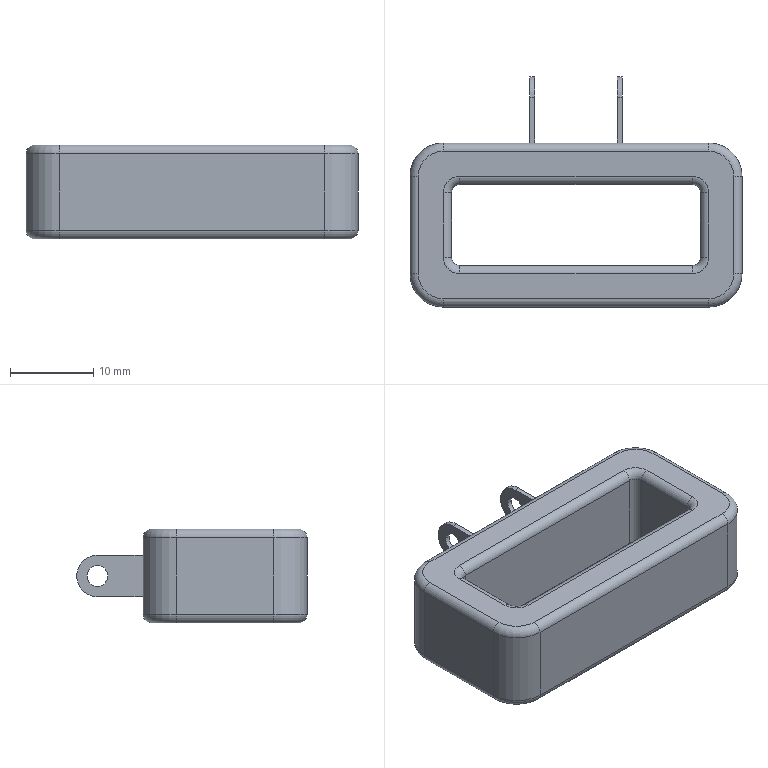Part | Creo | features CURVE 3, DATUM PLANE 3, PROTRUSION 2, ROUND 2, COORDINATE SYSTEM 1, CUT 1 | 1 solid | 64 faces | box 40 x 27.76 x 11.26 mm | volume 5415 mm3 | cylinder 30 | plane 18 | torus 16 | commonest cylinder face diameters 2 x20 2.5 x4 8 x4 5 x2